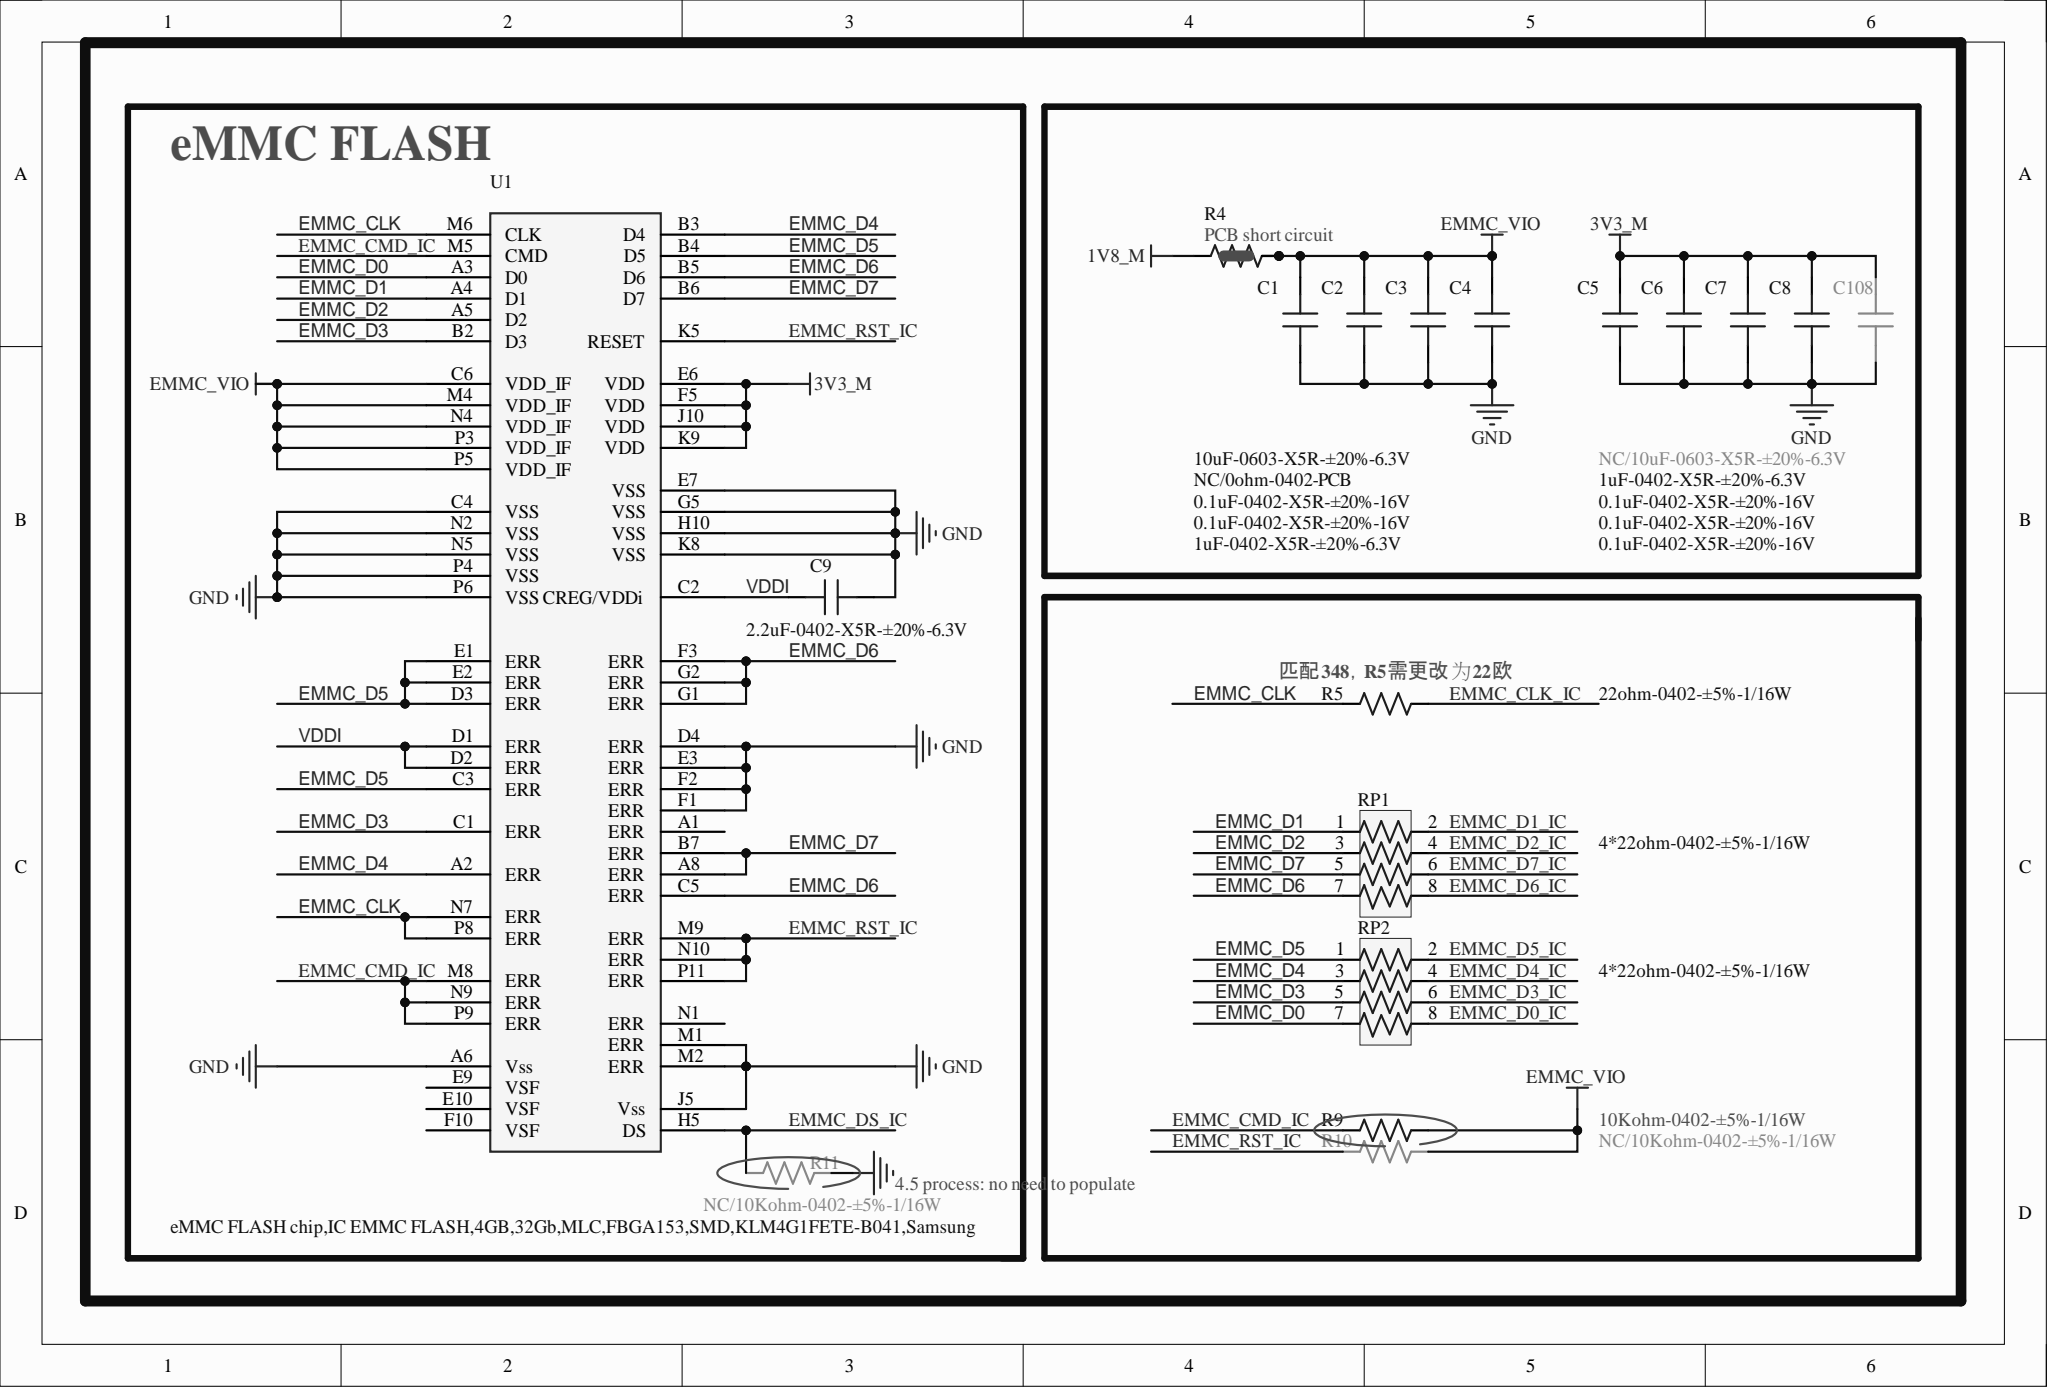Circuit board | Altium Designer | 951 parts | 509 nets | one sheet of the schematic
Parts on this sheet (reference | value | footprint):
C1 | 10uF-0603-X5R-±20%-6.3V | C0603
C2 | 1uF-0402-X5R-±20%-6.3V | C0402
C3 | 0.1uF-0402-X5R-±20%-16V | C0402
C4 | 0.1uF-0402-X5R-±20%-16V | C0402
C5 | 1uF-0402-X5R-±20%-6.3V | C0402
C8 | 0.1uF-0402-X5R-±20%-16V | C0402
C9 | 2.2uF-0402-X5R-±20%-6.3V | C0402
C108 | NC/10uF-0603-X5R-±20%-6.3V | C0603
R4 | NC/0ohm-0402-PCB | R0402SC
R5 | 22ohm-0402-±5%-1/16W | R0402
R9 | 10Kohm-0402-±5%-1/16W | R0402
R10 | NC/10Kohm-0402-±5%-1/16W | R0402
R11 | NC/10Kohm-0402-±5%-1/16W | R0402
RP1 | 4*22ohm-0402-±5%-1/16W | RA0402
RP2 | 4*22ohm-0402-±5%-1/16W | RA0402
U1 | eMMC FLASH chip,IC EMMC FLASH,4GB,32Gb,MLC,FBGA153,SMD,KLM4G1FETE-B041,Samsung | BGA153/0.5-1
Nets of these parts (net: part-pin ...):
VDDI: C9-1 U1-C2 U1-D1 U1-D2
GND: C1-1 C2-1 C3-1 C4-1 C5-1 C8-1 C9-2 C108-1 R11-1 U1-A6 U1-C4 U1-D4 U1-E3 U1-E7 U1-F1 U1-F2 U1-G5 U1-H10 U1-J5 U1-K8 U1-M1 U1-M2 U1-N2 U1-N5 U1-P4 U1-P6
EMMC_VIO: C1-2 C2-2 C3-2 C4-2 R4-2 R4-3 R9-2 R10-2 U1-C6 U1-M4 U1-N4 U1-P3 U1-P5
EMMC_RST_IC: R10-1 U1-K5 U1-M9 U1-N10 U1-P11
EMMC_DS_IC: R11-2 U1-H5
EMMC_D7_IC: RP1-6
EMMC_D7: RP1-5 U1-A8 U1-B6 U1-B7
EMMC_D6_IC: RP1-8
EMMC_D6: RP1-7 U1-B5 U1-C5 U1-F3 U1-G1 U1-G2
EMMC_D5_IC: RP2-2
EMMC_D5: RP2-1 U1-B4 U1-C3 U1-D3 U1-E1 U1-E2
EMMC_D4_IC: RP2-4
EMMC_D4: RP2-3 U1-A2 U1-B3
EMMC_D3_IC: RP2-6
EMMC_D3: RP2-5 U1-B2 U1-C1
EMMC_D2_IC: RP1-4
EMMC_D2: RP1-3 U1-A5
EMMC_D1_IC: RP1-2
EMMC_D1: RP1-1 U1-A4
EMMC_D0_IC: RP2-8
EMMC_D0: RP2-7 U1-A3
EMMC_CMD_IC: R9-1 U1-M5 U1-M8 U1-N9 U1-P9
EMMC_CLK_IC: R5-2
EMMC_CLK: R5-1 U1-M6 U1-N7 U1-P8
3V3_M: C5-2 C8-2 C108-2 U1-E6 U1-F5 U1-J10 U1-K9
1V8_M: R4-1